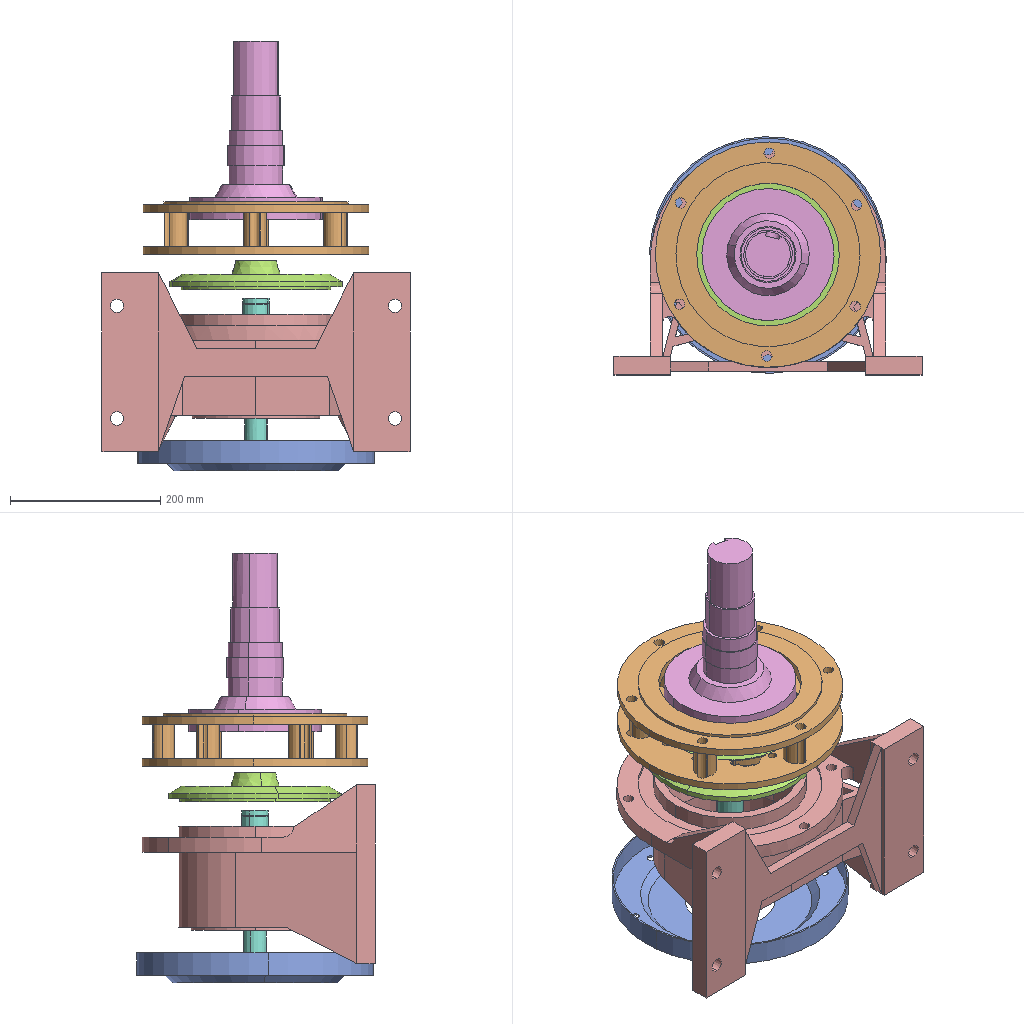Assembly | SolidWorks | 6 different items | 6 placed | box 410 x 317 x 572 mm
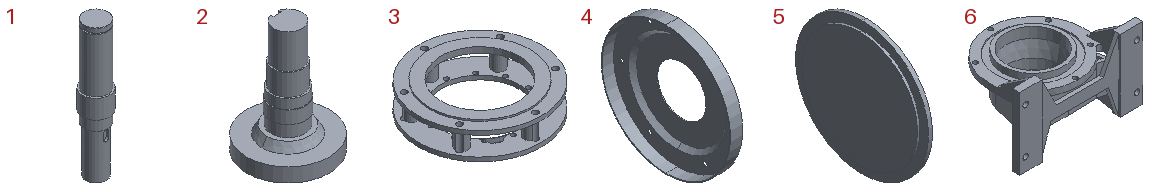Parts list (item | quantity | size | volume | features):
1 | x1 | 40 x 40 x 200 mm | 179024 mm3 | features ICE 8, Chamfer 1, Extrusion 1
2 | x1 | 176 x 176 x 238 mm | 1296573 mm3 | features ICE 10, Chamfer 1, Extrusion 1, Fillet 1
3 | x1 | 300 x 300 x 69.96 mm | 1053348 mm3 | features ICE 7, Extrusion 1
4 | x1 | 40 x 315 x 315 mm | 193331 mm3 | features ICE 2, Revolution 1, Shell 1
5 | x1 | 39 x 230 x 230 mm | 823549 mm3 | features Revolution 1
6 | x1 | 410 x 310 x 238 mm | 4128132 mm3 | features ICE 17, Fillet 5, Extrusion 1, MirrorPattern 1
Mates (type | each side: item.copy, entity, surface, feature):
Concentric | 6.1 face cone Cut-Extrude5 | 3.1 face cylinder Cut-Extrude3
Concentric | 6.1 face cylinder Cut-Extrude6 | 5.1 face cylinder Revolve1
Concentric | 2.1 face cylinder Boss-Extrude3 | 3.1 face cylinder Cut-Extrude3
Concentric | 6.1 face cylinder Cut-Extrude4 | 1.1 face cylinder Boss-Extrude1
Concentric | 6.1 face cylinder Boss-Extrude5 | 4.1 face cylinder Revolve1